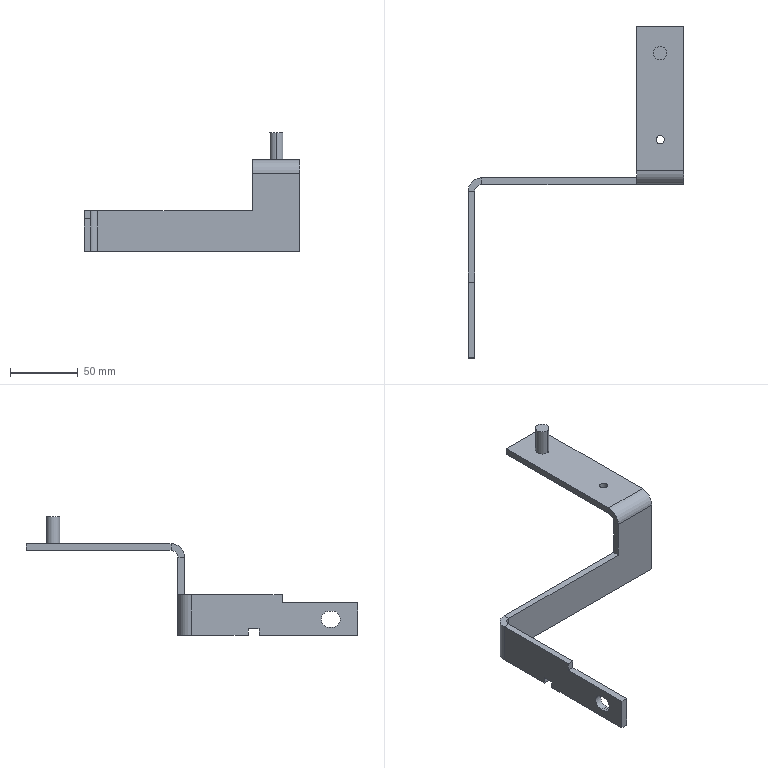Part | STEP file | 64560433 | 1 solid | 39 faces | box 159.4 x 245 x 87.7 mm | volume 67125 mm3 | plane 29 | cylinder 10 | commonest cylinder face diameters 10 x4 6 x2 12 x2 20 x2